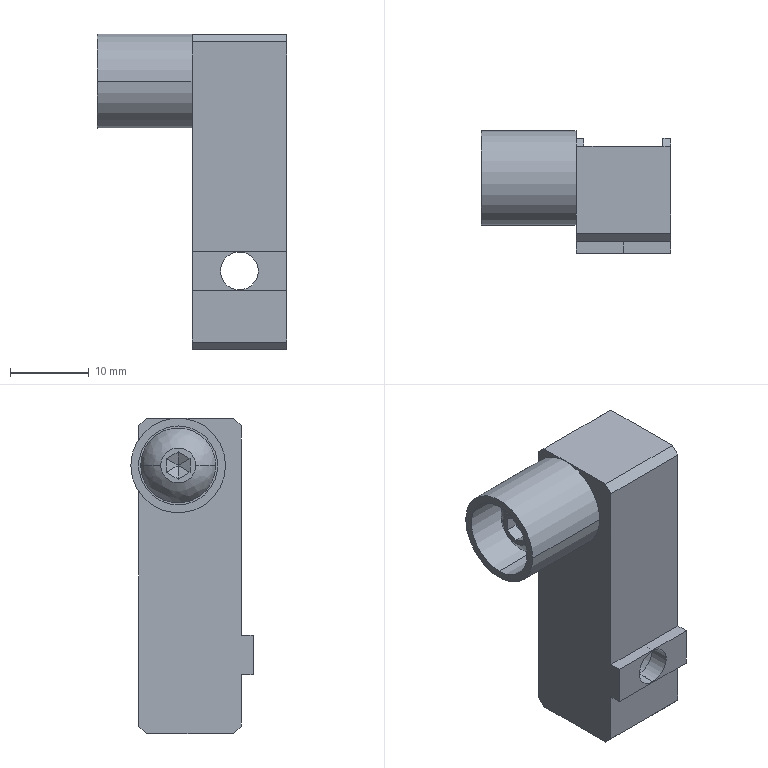Part | STEP file | Copy of hard limit assembly (right)^K50A-1H20-S(formula driven)-L300-motor left- | 3 solids | 59 faces | box 24 x 15.5 x 40 mm | volume 6072 mm3 | plane 39 | cylinder 16 | spline 2 | cone 2 | commonest cylinder face diameters 2.5 x2 4.2 x2 4.8 x2 5 x2 5.5 x2 9 x2